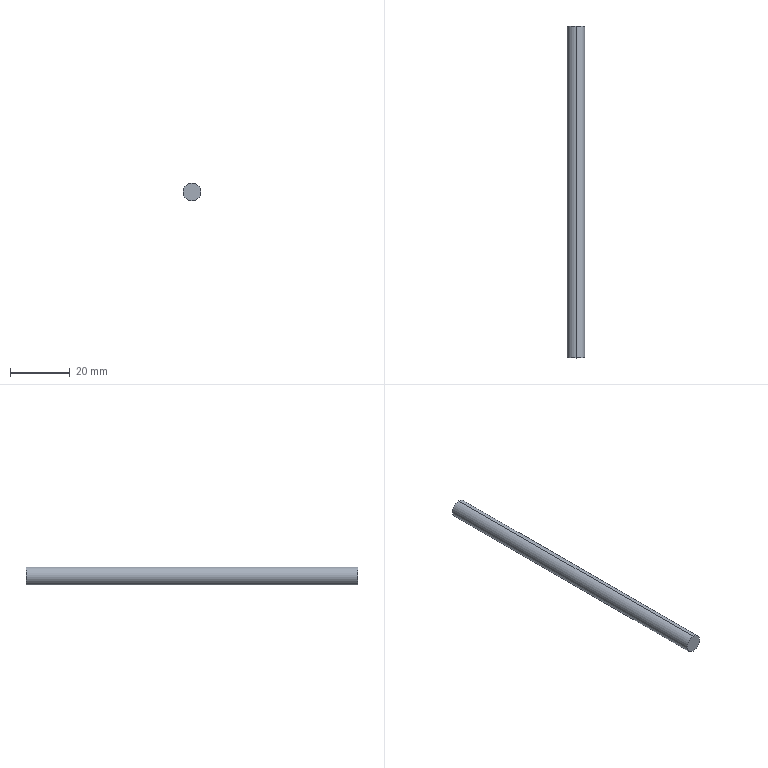Part | SolidWorks | features MirrorStock 1 | 1 solid | 4 faces | box 6 x 111.3 x 6 mm | volume 3147 mm3 | cylinder 2 | plane 2 | commonest cylinder face diameters 6 x2
STEP:
#1=CARTESIAN_POINT('',(0.,56.,-3.));
#2=VERTEX_POINT('',#1);
#3=CARTESIAN_POINT('',(0.,56.,3.));
#4=VERTEX_POINT('',#3);
#5=CARTESIAN_POINT('',(0.,56.,0.));
#6=DIRECTION('',(0.,1.,0.));
#7=DIRECTION('',(0.,0.,1.));
#8=AXIS2_PLACEMENT_3D('',#5,#6,#7);
#9=CIRCLE('',#8,3.);
#10=EDGE_CURVE('',#2,#4,#9,.T.);
#11=ORIENTED_EDGE('',*,*,#10,.F.);
#12=CARTESIAN_POINT('',(0.,-55.3,-3.));
#13=VERTEX_POINT('',#12);
#14=CARTESIAN_POINT('',(0.,-55.3,-3.));
#15=DIRECTION('',(0.,-1.,0.));
#16=VECTOR('',#15,1000.);
#17=LINE('',#14,#16);
#18=EDGE_CURVE('',#2,#13,#17,.T.);
#19=ORIENTED_EDGE('',*,*,#18,.T.);
#20=CARTESIAN_POINT('',(0.,-55.3,3.));
#21=VERTEX_POINT('',#20);
#22=CARTESIAN_POINT('',(0.,-55.3,0.));
#23=DIRECTION('',(0.,1.,0.));
#24=DIRECTION('',(0.,0.,1.));
#25=AXIS2_PLACEMENT_3D('',#22,#23,#24);
#26=CIRCLE('',#25,3.);
#27=EDGE_CURVE('',#13,#21,#26,.T.);
#28=ORIENTED_EDGE('',*,*,#27,.T.);
#29=CARTESIAN_POINT('',(0.,-55.3,3.));
#30=DIRECTION('',(0.,-1.,0.));
#31=VECTOR('',#30,1000.);
#32=LINE('',#29,#31);
#33=EDGE_CURVE('',#4,#21,#32,.T.);
#34=ORIENTED_EDGE('',*,*,#33,.F.);
#35=EDGE_LOOP('',(#11,#19,#28,#34));
#36=FACE_OUTER_BOUND('',#35,.T.);
#37=CARTESIAN_POINT('',(0.,-55.3,0.));
#38=DIRECTION('',(0.,-1.,0.));
#39=DIRECTION('',(0.,0.,1.));
#40=AXIS2_PLACEMENT_3D('',#37,#38,#39);
#41=CYLINDRICAL_SURFACE('',#40,3.);
#42=ADVANCED_FACE('',(#36),#41,.T.);
#43=CARTESIAN_POINT('',(0.,56.,0.));
#44=DIRECTION('',(0.,1.,0.));
#45=DIRECTION('',(0.,0.,1.));
#46=AXIS2_PLACEMENT_3D('',#43,#44,#45);
#47=CIRCLE('',#46,3.);
#48=EDGE_CURVE('',#4,#2,#47,.T.);
#49=ORIENTED_EDGE('',*,*,#48,.T.);
#50=ORIENTED_EDGE('',*,*,#10,.T.);
#51=EDGE_LOOP('',(#49,#50));
#52=FACE_OUTER_BOUND('',#51,.T.);
#53=CARTESIAN_POINT('',(0.,56.,0.));
#54=DIRECTION('',(0.,-1.,0.));
#55=DIRECTION('',(0.,0.,1.));
#56=AXIS2_PLACEMENT_3D('',#53,#54,#55);
#57=PLANE('',#56);
#58=ADVANCED_FACE('',(#52),#57,.F.);
#59=ORIENTED_EDGE('',*,*,#18,.F.);
#60=ORIENTED_EDGE('',*,*,#48,.F.);
#61=ORIENTED_EDGE('',*,*,#33,.T.);
#62=CARTESIAN_POINT('',(0.,-55.3,0.));
#63=DIRECTION('',(0.,1.,0.));
#64=DIRECTION('',(0.,0.,1.));
#65=AXIS2_PLACEMENT_3D('',#62,#63,#64);
#66=CIRCLE('',#65,3.);
#67=EDGE_CURVE('',#21,#13,#66,.T.);
#68=ORIENTED_EDGE('',*,*,#67,.T.);
#69=EDGE_LOOP('',(#59,#60,#61,#68));
#70=FACE_OUTER_BOUND('',#69,.T.);
#71=CARTESIAN_POINT('',(0.,-55.3,0.));
#72=DIRECTION('',(0.,-1.,0.));
#73=DIRECTION('',(0.,0.,1.));
#74=AXIS2_PLACEMENT_3D('',#71,#72,#73);
#75=CYLINDRICAL_SURFACE('',#74,3.);
#76=ADVANCED_FACE('',(#70),#75,.T.);
#77=ORIENTED_EDGE('',*,*,#67,.F.);
#78=ORIENTED_EDGE('',*,*,#27,.F.);
#79=EDGE_LOOP('',(#77,#78));
#80=FACE_OUTER_BOUND('',#79,.T.);
#81=CARTESIAN_POINT('',(3.,-55.3,0.));
#82=DIRECTION('',(0.,1.,0.));
#83=DIRECTION('',(0.,0.,-1.));
#84=AXIS2_PLACEMENT_3D('',#81,#82,#83);
#85=PLANE('',#84);
#86=ADVANCED_FACE('',(#80),#85,.F.);
#87=CLOSED_SHELL('',(#42,#58,#76,#86));
#88=MANIFOLD_SOLID_BREP('',#87);
#89=CARTESIAN_POINT('',(0.,0.,0.));
#90=DIRECTION('',(0.,0.,1.));
#91=DIRECTION('',(1.,0.,0.));
#92=AXIS2_PLACEMENT_3D('',#89,#90,#91);
#93=(LENGTH_UNIT()NAMED_UNIT(*)SI_UNIT(.MILLI.,.METRE.));
#94=UNCERTAINTY_MEASURE_WITH_UNIT(LENGTH_MEASURE(0.00001),#93,'','');
#95=(NAMED_UNIT(*)PLANE_ANGLE_UNIT()SI_UNIT($,.RADIAN.));
#96=(NAMED_UNIT(*)SI_UNIT($,.STERADIAN.)SOLID_ANGLE_UNIT());
#97=(GEOMETRIC_REPRESENTATION_CONTEXT(3)GLOBAL_UNCERTAINTY_ASSIGNED_CONTEXT((#94))GLOBAL_UNIT_ASSIGNED_CONTEXT((#93,#95,#96))REPRESENTATION_CONTEXT('',''));
#98=ADVANCED_BREP_SHAPE_REPRESENTATION('',(#88,#92),#97);